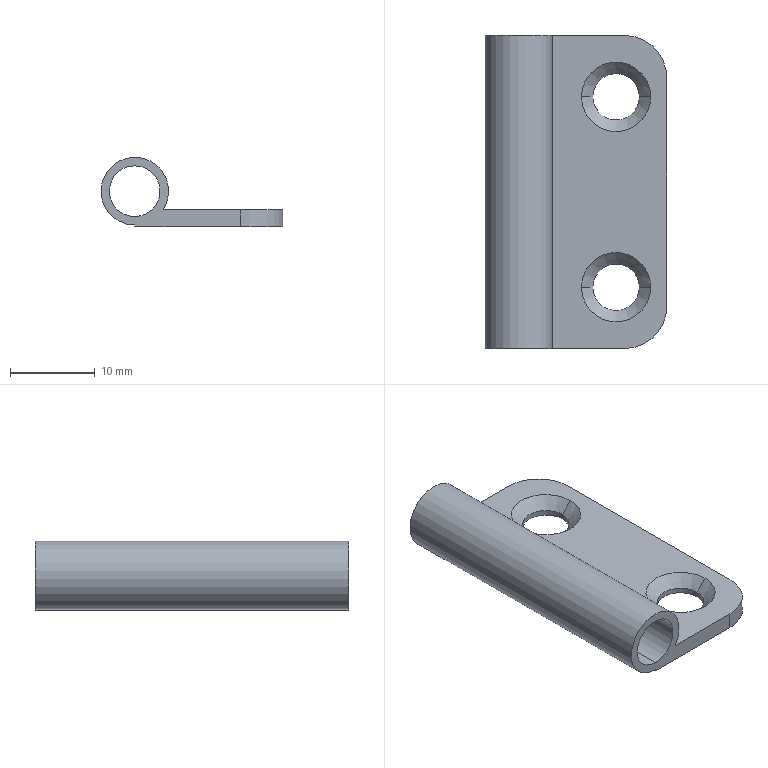Part | STEP file | heye1 | 1 solid | 19 faces | box 21.5 x 37 x 8.2 mm | volume 1799 mm3 | cylinder 9 | plane 6 | cone 4 | commonest cylinder face diameters 5.5 x4 6 x2 10 x2 8 x1
STEP:
#1=CARTESIAN_POINT('',(0.,0.,0.));
#2=DIRECTION('',(0.,0.,1.));
#3=DIRECTION('',(1.,0.,0.));
#4=AXIS2_PLACEMENT_3D('',#1,#2,#3);
#5=CARTESIAN_POINT('',(5.5,11.25,0.65));
#6=VERTEX_POINT('',#5);
#7=CARTESIAN_POINT('',(6.85,11.25,2.));
#8=VERTEX_POINT('',#7);
#9=CARTESIAN_POINT('',(6.85,11.25,2.));
#10=DIRECTION('',(0.7071,0.,0.7071));
#11=VECTOR('',#10,1.);
#12=LINE('',#9,#11);
#13=CARTESIAN_POINT('',(2.75,11.25,2.));
#14=DIRECTION('',(0.,0.,1.));
#15=DIRECTION('',(1.,0.,0.));
#16=AXIS2_PLACEMENT_3D('',#13,#14,#15);
#17=CONICAL_SURFACE('',#16,4.1,0.7854);
#18=CARTESIAN_POINT('',(6.283,0.));
#19=DIRECTION('',(0.,1.));
#20=VECTOR('',#19,1.);
#21=LINE('',#18,#20);
#22=(GEOMETRIC_REPRESENTATION_CONTEXT(2)PARAMETRIC_REPRESENTATION_CONTEXT()REPRESENTATION_CONTEXT('',''));
#23=DEFINITIONAL_REPRESENTATION('',(#21),#22);
#24=PCURVE('',#17,#23);
#25=CARTESIAN_POINT('',(2.75,11.25,2.));
#26=DIRECTION('',(0.,0.,1.));
#27=DIRECTION('',(1.,0.,0.));
#28=AXIS2_PLACEMENT_3D('',#25,#26,#27);
#29=CONICAL_SURFACE('',#28,4.1,0.7854);
#30=CARTESIAN_POINT('',(0.,0.));
#31=DIRECTION('',(0.,1.));
#32=VECTOR('',#31,1.);
#33=LINE('',#30,#32);
#34=(GEOMETRIC_REPRESENTATION_CONTEXT(2)PARAMETRIC_REPRESENTATION_CONTEXT()REPRESENTATION_CONTEXT('',''));
#35=DEFINITIONAL_REPRESENTATION('',(#33),#34);
#36=PCURVE('',#29,#35);
#37=SURFACE_CURVE('',#12,(#24,#36),.PCURVE_S1.);
#38=EDGE_CURVE('',#6,#8,#37,.T.);
#39=ORIENTED_EDGE('',*,*,#38,.T.);
#40=CARTESIAN_POINT('',(-1.35,11.25,2.));
#41=VERTEX_POINT('',#40);
#42=CARTESIAN_POINT('',(2.75,11.25,2.));
#43=DIRECTION('',(0.,0.,1.));
#44=DIRECTION('',(1.,0.,0.));
#45=AXIS2_PLACEMENT_3D('',#42,#43,#44);
#46=CIRCLE('',#45,4.1);
#47=CARTESIAN_POINT('',(0.,0.));
#48=DIRECTION('',(1.,0.));
#49=VECTOR('',#48,1.);
#50=LINE('',#47,#49);
#51=(GEOMETRIC_REPRESENTATION_CONTEXT(2)PARAMETRIC_REPRESENTATION_CONTEXT()REPRESENTATION_CONTEXT('',''));
#52=DEFINITIONAL_REPRESENTATION('',(#50),#51);
#53=PCURVE('',#17,#52);
#54=CARTESIAN_POINT('',(0.,0.,2.));
#55=DIRECTION('',(0.,0.,-1.));
#56=DIRECTION('',(-1.,0.,0.));
#57=AXIS2_PLACEMENT_3D('',#54,#55,#56);
#58=PLANE('',#57);
#59=CARTESIAN_POINT('',(-6.85,11.25));
#60=CARTESIAN_POINT('',(-6.85,18.351));
#61=CARTESIAN_POINT('',(-0.7,14.801));
#62=CARTESIAN_POINT('',(5.45,11.25));
#63=CARTESIAN_POINT('',(-0.7,7.699));
#64=CARTESIAN_POINT('',(-6.85,4.149));
#65=CARTESIAN_POINT('',(-6.85,11.25));
#66=(BOUNDED_CURVE()B_SPLINE_CURVE(2,(#59,#60,#61,#62,#63,#64,#65),.UNSPECIFIED.,.T.,.F.)B_SPLINE_CURVE_WITH_KNOTS((1,2,2,2,2,1),(-2.094,0.,2.094,4.189,6.283,8.378),.UNSPECIFIED.)CURVE()GEOMETRIC_REPRESENTATION_ITEM()RATIONAL_B_SPLINE_CURVE((1.,0.5,1.,0.5,1.,0.5,1.))REPRESENTATION_ITEM(''));
#67=(GEOMETRIC_REPRESENTATION_CONTEXT(2)PARAMETRIC_REPRESENTATION_CONTEXT()REPRESENTATION_CONTEXT('',''));
#68=DEFINITIONAL_REPRESENTATION('',(#66),#67);
#69=PCURVE('',#58,#68);
#70=SURFACE_CURVE('',#46,(#53,#69),.PCURVE_S1.);
#71=EDGE_CURVE('',#41,#8,#70,.T.);
#72=ORIENTED_EDGE('',*,*,#71,.F.);
#73=CARTESIAN_POINT('',(0.,11.25,0.65));
#74=VERTEX_POINT('',#73);
#75=CARTESIAN_POINT('',(-1.35,11.25,2.));
#76=DIRECTION('',(-0.7071,0.,0.7071));
#77=VECTOR('',#76,1.);
#78=LINE('',#75,#77);
#79=CARTESIAN_POINT('',(3.142,0.));
#80=DIRECTION('',(0.,1.));
#81=VECTOR('',#80,1.);
#82=LINE('',#79,#81);
#83=(GEOMETRIC_REPRESENTATION_CONTEXT(2)PARAMETRIC_REPRESENTATION_CONTEXT()REPRESENTATION_CONTEXT('',''));
#84=DEFINITIONAL_REPRESENTATION('',(#82),#83);
#85=PCURVE('',#17,#84);
#86=CARTESIAN_POINT('',(3.142,0.));
#87=DIRECTION('',(0.,1.));
#88=VECTOR('',#87,1.);
#89=LINE('',#86,#88);
#90=(GEOMETRIC_REPRESENTATION_CONTEXT(2)PARAMETRIC_REPRESENTATION_CONTEXT()REPRESENTATION_CONTEXT('',''));
#91=DEFINITIONAL_REPRESENTATION('',(#89),#90);
#92=PCURVE('',#29,#91);
#93=SURFACE_CURVE('',#78,(#85,#92),.PCURVE_S1.);
#94=EDGE_CURVE('',#74,#41,#93,.T.);
#95=ORIENTED_EDGE('',*,*,#94,.F.);
#96=CARTESIAN_POINT('',(2.75,11.25,0.65));
#97=DIRECTION('',(0.,0.,1.));
#98=DIRECTION('',(1.,0.,0.));
#99=AXIS2_PLACEMENT_3D('',#96,#97,#98);
#100=CIRCLE('',#99,2.75);
#101=CARTESIAN_POINT('',(0.,-1.35));
#102=DIRECTION('',(1.,0.));
#103=VECTOR('',#102,1.);
#104=LINE('',#101,#103);
#105=(GEOMETRIC_REPRESENTATION_CONTEXT(2)PARAMETRIC_REPRESENTATION_CONTEXT()REPRESENTATION_CONTEXT('',''));
#106=DEFINITIONAL_REPRESENTATION('',(#104),#105);
#107=PCURVE('',#17,#106);
#108=CARTESIAN_POINT('',(2.75,11.25,2.));
#109=DIRECTION('',(0.,0.,1.));
#110=DIRECTION('',(1.,0.,0.));
#111=AXIS2_PLACEMENT_3D('',#108,#109,#110);
#112=CYLINDRICAL_SURFACE('',#111,2.75);
#113=CARTESIAN_POINT('',(0.,-1.35));
#114=DIRECTION('',(1.,0.));
#115=VECTOR('',#114,1.);
#116=LINE('',#113,#115);
#117=(GEOMETRIC_REPRESENTATION_CONTEXT(2)PARAMETRIC_REPRESENTATION_CONTEXT()REPRESENTATION_CONTEXT('',''));
#118=DEFINITIONAL_REPRESENTATION('',(#116),#117);
#119=PCURVE('',#112,#118);
#120=SURFACE_CURVE('',#100,(#107,#119),.PCURVE_S1.);
#121=EDGE_CURVE('',#74,#6,#120,.T.);
#122=ORIENTED_EDGE('',*,*,#121,.T.);
#123=EDGE_LOOP('',(#39,#72,#95,#122));
#124=FACE_BOUND('',#123,.F.);
#125=ADVANCED_FACE('',(#124),#17,.F.);
#126=CARTESIAN_POINT('',(5.5,11.25,0.));
#127=VERTEX_POINT('',#126);
#128=CARTESIAN_POINT('',(5.5,11.25,2.));
#129=DIRECTION('',(0.,0.,1.));
#130=VECTOR('',#129,1.);
#131=LINE('',#128,#130);
#132=CARTESIAN_POINT('',(6.283,0.));
#133=DIRECTION('',(0.,1.));
#134=VECTOR('',#133,1.);
#135=LINE('',#132,#134);
#136=(GEOMETRIC_REPRESENTATION_CONTEXT(2)PARAMETRIC_REPRESENTATION_CONTEXT()REPRESENTATION_CONTEXT('',''));
#137=DEFINITIONAL_REPRESENTATION('',(#135),#136);
#138=PCURVE('',#112,#137);
#139=CARTESIAN_POINT('',(2.75,11.25,2.));
#140=DIRECTION('',(0.,0.,1.));
#141=DIRECTION('',(1.,0.,0.));
#142=AXIS2_PLACEMENT_3D('',#139,#140,#141);
#143=CYLINDRICAL_SURFACE('',#142,2.75);
#144=CARTESIAN_POINT('',(0.,0.));
#145=DIRECTION('',(0.,1.));
#146=VECTOR('',#145,1.);
#147=LINE('',#144,#146);
#148=(GEOMETRIC_REPRESENTATION_CONTEXT(2)PARAMETRIC_REPRESENTATION_CONTEXT()REPRESENTATION_CONTEXT('',''));
#149=DEFINITIONAL_REPRESENTATION('',(#147),#148);
#150=PCURVE('',#143,#149);
#151=SURFACE_CURVE('',#131,(#138,#150),.PCURVE_S1.);
#152=EDGE_CURVE('',#127,#6,#151,.T.);
#153=ORIENTED_EDGE('',*,*,#152,.T.);
#154=ORIENTED_EDGE('',*,*,#121,.F.);
#155=CARTESIAN_POINT('',(0.,11.25,0.));
#156=VERTEX_POINT('',#155);
#157=CARTESIAN_POINT('',(0.,11.25,2.));
#158=DIRECTION('',(0.,0.,1.));
#159=VECTOR('',#158,1.);
#160=LINE('',#157,#159);
#161=CARTESIAN_POINT('',(3.142,0.));
#162=DIRECTION('',(0.,1.));
#163=VECTOR('',#162,1.);
#164=LINE('',#161,#163);
#165=(GEOMETRIC_REPRESENTATION_CONTEXT(2)PARAMETRIC_REPRESENTATION_CONTEXT()REPRESENTATION_CONTEXT('',''));
#166=DEFINITIONAL_REPRESENTATION('',(#164),#165);
#167=PCURVE('',#112,#166);
#168=CARTESIAN_POINT('',(3.142,0.));
#169=DIRECTION('',(0.,1.));
#170=VECTOR('',#169,1.);
#171=LINE('',#168,#170);
#172=(GEOMETRIC_REPRESENTATION_CONTEXT(2)PARAMETRIC_REPRESENTATION_CONTEXT()REPRESENTATION_CONTEXT('',''));
#173=DEFINITIONAL_REPRESENTATION('',(#171),#172);
#174=PCURVE('',#143,#173);
#175=SURFACE_CURVE('',#160,(#167,#174),.PCURVE_S1.);
#176=EDGE_CURVE('',#156,#74,#175,.T.);
#177=ORIENTED_EDGE('',*,*,#176,.F.);
#178=CARTESIAN_POINT('',(2.75,11.25,0.));
#179=DIRECTION('',(0.,0.,1.));
#180=DIRECTION('',(1.,0.,0.));
#181=AXIS2_PLACEMENT_3D('',#178,#179,#180);
#182=CIRCLE('',#181,2.75);
#183=CARTESIAN_POINT('',(0.,-2.));
#184=DIRECTION('',(1.,0.));
#185=VECTOR('',#184,1.);
#186=LINE('',#183,#185);
#187=(GEOMETRIC_REPRESENTATION_CONTEXT(2)PARAMETRIC_REPRESENTATION_CONTEXT()REPRESENTATION_CONTEXT('',''));
#188=DEFINITIONAL_REPRESENTATION('',(#186),#187);
#189=PCURVE('',#112,#188);
#190=CARTESIAN_POINT('',(0.,0.,0.));
#191=DIRECTION('',(0.,0.,-1.));
#192=DIRECTION('',(-1.,0.,0.));
#193=AXIS2_PLACEMENT_3D('',#190,#191,#192);
#194=PLANE('',#193);
#195=CARTESIAN_POINT('',(-5.5,11.25));
#196=CARTESIAN_POINT('',(-5.5,16.013));
#197=CARTESIAN_POINT('',(-1.375,13.632));
#198=CARTESIAN_POINT('',(2.75,11.25));
#199=CARTESIAN_POINT('',(-1.375,8.868));
#200=CARTESIAN_POINT('',(-5.5,6.487));
#201=CARTESIAN_POINT('',(-5.5,11.25));
#202=(BOUNDED_CURVE()B_SPLINE_CURVE(2,(#195,#196,#197,#198,#199,#200,#201),.UNSPECIFIED.,.T.,.F.)B_SPLINE_CURVE_WITH_KNOTS((1,2,2,2,2,1),(-2.094,0.,2.094,4.189,6.283,8.378),.UNSPECIFIED.)CURVE()GEOMETRIC_REPRESENTATION_ITEM()RATIONAL_B_SPLINE_CURVE((1.,0.5,1.,0.5,1.,0.5,1.))REPRESENTATION_ITEM(''));
#203=(GEOMETRIC_REPRESENTATION_CONTEXT(2)PARAMETRIC_REPRESENTATION_CONTEXT()REPRESENTATION_CONTEXT('',''));
#204=DEFINITIONAL_REPRESENTATION('',(#202),#203);
#205=PCURVE('',#194,#204);
#206=SURFACE_CURVE('',#182,(#189,#205),.PCURVE_S1.);
#207=EDGE_CURVE('',#156,#127,#206,.T.);
#208=ORIENTED_EDGE('',*,*,#207,.T.);
#209=EDGE_LOOP('',(#153,#154,#177,#208));
#210=FACE_BOUND('',#209,.F.);
#211=ADVANCED_FACE('',(#210),#112,.F.);
#212=CARTESIAN_POINT('',(5.5,-11.25,0.65));
#213=VERTEX_POINT('',#212);
#214=CARTESIAN_POINT('',(6.85,-11.25,2.));
#215=VERTEX_POINT('',#214);
#216=CARTESIAN_POINT('',(6.85,-11.25,2.));
#217=DIRECTION('',(0.7071,0.,0.7071));
#218=VECTOR('',#217,1.);
#219=LINE('',#216,#218);
#220=CARTESIAN_POINT('',(2.75,-11.25,2.));
#221=DIRECTION('',(0.,0.,1.));
#222=DIRECTION('',(1.,0.,0.));
#223=AXIS2_PLACEMENT_3D('',#220,#221,#222);
#224=CONICAL_SURFACE('',#223,4.1,0.7854);
#225=CARTESIAN_POINT('',(6.283,0.));
#226=DIRECTION('',(0.,1.));
#227=VECTOR('',#226,1.);
#228=LINE('',#225,#227);
#229=(GEOMETRIC_REPRESENTATION_CONTEXT(2)PARAMETRIC_REPRESENTATION_CONTEXT()REPRESENTATION_CONTEXT('',''));
#230=DEFINITIONAL_REPRESENTATION('',(#228),#229);
#231=PCURVE('',#224,#230);
#232=CARTESIAN_POINT('',(2.75,-11.25,2.));
#233=DIRECTION('',(0.,0.,1.));
#234=DIRECTION('',(1.,0.,0.));
#235=AXIS2_PLACEMENT_3D('',#232,#233,#234);
#236=CONICAL_SURFACE('',#235,4.1,0.7854);
#237=CARTESIAN_POINT('',(0.,0.));
#238=DIRECTION('',(0.,1.));
#239=VECTOR('',#238,1.);
#240=LINE('',#237,#239);
#241=(GEOMETRIC_REPRESENTATION_CONTEXT(2)PARAMETRIC_REPRESENTATION_CONTEXT()REPRESENTATION_CONTEXT('',''));
#242=DEFINITIONAL_REPRESENTATION('',(#240),#241);
#243=PCURVE('',#236,#242);
#244=SURFACE_CURVE('',#219,(#231,#243),.PCURVE_S1.);
#245=EDGE_CURVE('',#213,#215,#244,.T.);
#246=ORIENTED_EDGE('',*,*,#245,.T.);
#247=CARTESIAN_POINT('',(-1.35,-11.25,2.));
#248=VERTEX_POINT('',#247);
#249=CARTESIAN_POINT('',(2.75,-11.25,2.));
#250=DIRECTION('',(0.,0.,1.));
#251=DIRECTION('',(1.,0.,0.));
#252=AXIS2_PLACEMENT_3D('',#249,#250,#251);
#253=CIRCLE('',#252,4.1);
#254=CARTESIAN_POINT('',(0.,0.));
#255=DIRECTION('',(1.,0.));
#256=VECTOR('',#255,1.);
#257=LINE('',#254,#256);
#258=(GEOMETRIC_REPRESENTATION_CONTEXT(2)PARAMETRIC_REPRESENTATION_CONTEXT()REPRESENTATION_CONTEXT('',''));
#259=DEFINITIONAL_REPRESENTATION('',(#257),#258);
#260=PCURVE('',#224,#259);
#261=CARTESIAN_POINT('',(-6.85,-11.25));
#262=CARTESIAN_POINT('',(-6.85,-4.149));
#263=CARTESIAN_POINT('',(-0.7,-7.699));
#264=CARTESIAN_POINT('',(5.45,-11.25));
#265=CARTESIAN_POINT('',(-0.7,-14.801));
#266=CARTESIAN_POINT('',(-6.85,-18.351));
#267=CARTESIAN_POINT('',(-6.85,-11.25));
#268=(BOUNDED_CURVE()B_SPLINE_CURVE(2,(#261,#262,#263,#264,#265,#266,#267),.UNSPECIFIED.,.T.,.F.)B_SPLINE_CURVE_WITH_KNOTS((1,2,2,2,2,1),(-2.094,0.,2.094,4.189,6.283,8.378),.UNSPECIFIED.)CURVE()GEOMETRIC_REPRESENTATION_ITEM()RATIONAL_B_SPLINE_CURVE((1.,0.5,1.,0.5,1.,0.5,1.))REPRESENTATION_ITEM(''));
#269=(GEOMETRIC_REPRESENTATION_CONTEXT(2)PARAMETRIC_REPRESENTATION_CONTEXT()REPRESENTATION_CONTEXT('',''));
#270=DEFINITIONAL_REPRESENTATION('',(#268),#269);
#271=PCURVE('',#58,#270);
#272=SURFACE_CURVE('',#253,(#260,#271),.PCURVE_S1.);
#273=EDGE_CURVE('',#248,#215,#272,.T.);
#274=ORIENTED_EDGE('',*,*,#273,.F.);
#275=CARTESIAN_POINT('',(0.,-11.25,0.65));
#276=VERTEX_POINT('',#275);
#277=CARTESIAN_POINT('',(-1.35,-11.25,2.));
#278=DIRECTION('',(-0.7071,0.,0.7071));
#279=VECTOR('',#278,1.);
#280=LINE('',#277,#279);
#281=CARTESIAN_POINT('',(3.142,0.));
#282=DIRECTION('',(0.,1.));
#283=VECTOR('',#282,1.);
#284=LINE('',#281,#283);
#285=(GEOMETRIC_REPRESENTATION_CONTEXT(2)PARAMETRIC_REPRESENTATION_CONTEXT()REPRESENTATION_CONTEXT('',''));
#286=DEFINITIONAL_REPRESENTATION('',(#284),#285);
#287=PCURVE('',#224,#286);
#288=CARTESIAN_POINT('',(3.142,0.));
#289=DIRECTION('',(0.,1.));
#290=VECTOR('',#289,1.);
#291=LINE('',#288,#290);
#292=(GEOMETRIC_REPRESENTATION_CONTEXT(2)PARAMETRIC_REPRESENTATION_CONTEXT()REPRESENTATION_CONTEXT('',''));
#293=DEFINITIONAL_REPRESENTATION('',(#291),#292);
#294=PCURVE('',#236,#293);
#295=SURFACE_CURVE('',#280,(#287,#294),.PCURVE_S1.);
#296=EDGE_CURVE('',#276,#248,#295,.T.);
#297=ORIENTED_EDGE('',*,*,#296,.F.);
#298=CARTESIAN_POINT('',(2.75,-11.25,0.65));
#299=DIRECTION('',(0.,0.,1.));
#300=DIRECTION('',(1.,0.,0.));
#301=AXIS2_PLACEMENT_3D('',#298,#299,#300);
#302=CIRCLE('',#301,2.75);
#303=CARTESIAN_POINT('',(0.,-1.35));
#304=DIRECTION('',(1.,0.));
#305=VECTOR('',#304,1.);
#306=LINE('',#303,#305);
#307=(GEOMETRIC_REPRESENTATION_CONTEXT(2)PARAMETRIC_REPRESENTATION_CONTEXT()REPRESENTATION_CONTEXT('',''));
#308=DEFINITIONAL_REPRESENTATION('',(#306),#307);
#309=PCURVE('',#224,#308);
#310=CARTESIAN_POINT('',(2.75,-11.25,2.));
#311=DIRECTION('',(0.,0.,1.));
#312=DIRECTION('',(1.,0.,0.));
#313=AXIS2_PLACEMENT_3D('',#310,#311,#312);
#314=CYLINDRICAL_SURFACE('',#313,2.75);
#315=CARTESIAN_POINT('',(0.,-1.35));
#316=DIRECTION('',(1.,0.));
#317=VECTOR('',#316,1.);
#318=LINE('',#315,#317);
#319=(GEOMETRIC_REPRESENTATION_CONTEXT(2)PARAMETRIC_REPRESENTATION_CONTEXT()REPRESENTATION_CONTEXT('',''));
#320=DEFINITIONAL_REPRESENTATION('',(#318),#319);
#321=PCURVE('',#314,#320);
#322=SURFACE_CURVE('',#302,(#309,#321),.PCURVE_S1.);
#323=EDGE_CURVE('',#276,#213,#322,.T.);
#324=ORIENTED_EDGE('',*,*,#323,.T.);
#325=EDGE_LOOP('',(#246,#274,#297,#324));
#326=FACE_BOUND('',#325,.F.);
#327=ADVANCED_FACE('',(#326),#224,.F.);
#328=CARTESIAN_POINT('',(5.5,-11.25,0.));
#329=VERTEX_POINT('',#328);
#330=CARTESIAN_POINT('',(5.5,-11.25,2.));
#331=DIRECTION('',(0.,0.,1.));
#332=VECTOR('',#331,1.);
#333=LINE('',#330,#332);
#334=CARTESIAN_POINT('',(6.283,0.));
#335=DIRECTION('',(0.,1.));
#336=VECTOR('',#335,1.);
#337=LINE('',#334,#336);
#338=(GEOMETRIC_REPRESENTATION_CONTEXT(2)PARAMETRIC_REPRESENTATION_CONTEXT()REPRESENTATION_CONTEXT('',''));
#339=DEFINITIONAL_REPRESENTATION('',(#337),#338);
#340=PCURVE('',#314,#339);
#341=CARTESIAN_POINT('',(2.75,-11.25,2.));
#342=DIRECTION('',(0.,0.,1.));
#343=DIRECTION('',(1.,0.,0.));
#344=AXIS2_PLACEMENT_3D('',#341,#342,#343);
#345=CYLINDRICAL_SURFACE('',#344,2.75);
#346=CARTESIAN_POINT('',(0.,0.));
#347=DIRECTION('',(0.,1.));
#348=VECTOR('',#347,1.);
#349=LINE('',#346,#348);
#350=(GEOMETRIC_REPRESENTATION_CONTEXT(2)PARAMETRIC_REPRESENTATION_CONTEXT()REPRESENTATION_CONTEXT('',''));
#351=DEFINITIONAL_REPRESENTATION('',(#349),#350);
#352=PCURVE('',#345,#351);
#353=SURFACE_CURVE('',#333,(#340,#352),.PCURVE_S1.);
#354=EDGE_CURVE('',#329,#213,#353,.T.);
#355=ORIENTED_EDGE('',*,*,#354,.T.);
#356=ORIENTED_EDGE('',*,*,#323,.F.);
#357=CARTESIAN_POINT('',(0.,-11.25,0.));
#358=VERTEX_POINT('',#357);
#359=CARTESIAN_POINT('',(0.,-11.25,2.));
#360=DIRECTION('',(0.,0.,1.));
#361=VECTOR('',#360,1.);
#362=LINE('',#359,#361);
#363=CARTESIAN_POINT('',(3.142,0.));
#364=DIRECTION('',(0.,1.));
#365=VECTOR('',#364,1.);
#366=LINE('',#363,#365);
#367=(GEOMETRIC_REPRESENTATION_CONTEXT(2)PARAMETRIC_REPRESENTATION_CONTEXT()REPRESENTATION_CONTEXT('',''));
#368=DEFINITIONAL_REPRESENTATION('',(#366),#367);
#369=PCURVE('',#314,#368);
#370=CARTESIAN_POINT('',(3.142,0.));
#371=DIRECTION('',(0.,1.));
#372=VECTOR('',#371,1.);
#373=LINE('',#370,#372);
#374=(GEOMETRIC_REPRESENTATION_CONTEXT(2)PARAMETRIC_REPRESENTATION_CONTEXT()REPRESENTATION_CONTEXT('',''));
#375=DEFINITIONAL_REPRESENTATION('',(#373),#374);
#376=PCURVE('',#345,#375);
#377=SURFACE_CURVE('',#362,(#369,#376),.PCURVE_S1.);
#378=EDGE_CURVE('',#358,#276,#377,.T.);
#379=ORIENTED_EDGE('',*,*,#378,.F.);
#380=CARTESIAN_POINT('',(2.75,-11.25,0.));
#381=DIRECTION('',(0.,0.,1.));
#382=DIRECTION('',(1.,0.,0.));
#383=AXIS2_PLACEMENT_3D('',#380,#381,#382);
#384=CIRCLE('',#383,2.75);
#385=CARTESIAN_POINT('',(0.,-2.));
#386=DIRECTION('',(1.,0.));
#387=VECTOR('',#386,1.);
#388=LINE('',#385,#387);
#389=(GEOMETRIC_REPRESENTATION_CONTEXT(2)PARAMETRIC_REPRESENTATION_CONTEXT()REPRESENTATION_CONTEXT('',''));
#390=DEFINITIONAL_REPRESENTATION('',(#388),#389);
#391=PCURVE('',#314,#390);
#392=CARTESIAN_POINT('',(-5.5,-11.25));
#393=CARTESIAN_POINT('',(-5.5,-6.487));
#394=CARTESIAN_POINT('',(-1.375,-8.868));
#395=CARTESIAN_POINT('',(2.75,-11.25));
#396=CARTESIAN_POINT('',(-1.375,-13.632));
#397=CARTESIAN_POINT('',(-5.5,-16.013));
#398=CARTESIAN_POINT('',(-5.5,-11.25));
#399=(BOUNDED_CURVE()B_SPLINE_CURVE(2,(#392,#393,#394,#395,#396,#397,#398),.UNSPECIFIED.,.T.,.F.)B_SPLINE_CURVE_WITH_KNOTS((1,2,2,2,2,1),(-2.094,0.,2.094,4.189,6.283,8.378),.UNSPECIFIED.)CURVE()GEOMETRIC_REPRESENTATION_ITEM()RATIONAL_B_SPLINE_CURVE((1.,0.5,1.,0.5,1.,0.5,1.))REPRESENTATION_ITEM(''));
#400=(GEOMETRIC_REPRESENTATION_CONTEXT(2)PARAMETRIC_REPRESENTATION_CONTEXT()REPRESENTATION_CONTEXT('',''));
#401=DEFINITIONAL_REPRESENTATION('',(#399),#400);
#402=PCURVE('',#194,#401);
#403=SURFACE_CURVE('',#384,(#391,#402),.PCURVE_S1.);
#404=EDGE_CURVE('',#358,#329,#403,.T.);
#405=ORIENTED_EDGE('',*,*,#404,.T.);
#406=EDGE_LOOP('',(#355,#356,#379,#405));
#407=FACE_BOUND('',#406,.F.);
#408=ADVANCED_FACE('',(#407),#314,.F.);
#409=CARTESIAN_POINT('',(-8.75,-18.5,7.2));
#410=VERTEX_POINT('',#409);
#411=CARTESIAN_POINT('',(-8.75,18.5,7.2));
#412=VERTEX_POINT('',#411);
#413=CARTESIAN_POINT('',(-8.75,-18.5,7.2));
#414=DIRECTION('',(0.,1.,0.));
#415=VECTOR('',#414,1.);
#416=LINE('',#413,#415);
#417=CARTESIAN_POINT('',(-8.75,-18.5,4.2));
#418=DIRECTION('',(0.,1.,0.));
#419=DIRECTION('',(0.,0.,1.));
#420=AXIS2_PLACEMENT_3D('',#417,#418,#419);
#421=CYLINDRICAL_SURFACE('',#420,3.);
#422=CARTESIAN_POINT('',(6.283,0.));
#423=DIRECTION('',(0.,1.));
#424=VECTOR('',#423,1.);
#425=LINE('',#422,#424);
#426=(GEOMETRIC_REPRESENTATION_CONTEXT(2)PARAMETRIC_REPRESENTATION_CONTEXT()REPRESENTATION_CONTEXT('',''));
#427=DEFINITIONAL_REPRESENTATION('',(#425),#426);
#428=PCURVE('',#421,#427);
#429=CARTESIAN_POINT('',(-8.75,-18.5,4.2));
#430=DIRECTION('',(0.,1.,0.));
#431=DIRECTION('',(0.,0.,1.));
#432=AXIS2_PLACEMENT_3D('',#429,#430,#431);
#433=CYLINDRICAL_SURFACE('',#432,3.);
#434=CARTESIAN_POINT('',(0.,0.));
#435=DIRECTION('',(0.,1.));
#436=VECTOR('',#435,1.);
#437=LINE('',#434,#436);
#438=(GEOMETRIC_REPRESENTATION_CONTEXT(2)PARAMETRIC_REPRESENTATION_CONTEXT()REPRESENTATION_CONTEXT('',''));
#439=DEFINITIONAL_REPRESENTATION('',(#437),#438);
#440=PCURVE('',#433,#439);
#441=SURFACE_CURVE('',#416,(#428,#440),.PCURVE_S1.);
#442=EDGE_CURVE('',#410,#412,#441,.T.);
#443=ORIENTED_EDGE('',*,*,#442,.T.);
#444=CARTESIAN_POINT('',(-8.75,18.5,1.2));
#445=VERTEX_POINT('',#444);
#446=CARTESIAN_POINT('',(-8.75,18.5,4.2));
#447=DIRECTION('',(0.,1.,0.));
#448=DIRECTION('',(0.,0.,1.));
#449=AXIS2_PLACEMENT_3D('',#446,#447,#448);
#450=CIRCLE('',#449,3.);
#451=CARTESIAN_POINT('',(0.,37.));
#452=DIRECTION('',(1.,0.));
#453=VECTOR('',#452,1.);
#454=LINE('',#451,#453);
#455=(GEOMETRIC_REPRESENTATION_CONTEXT(2)PARAMETRIC_REPRESENTATION_CONTEXT()REPRESENTATION_CONTEXT('',''));
#456=DEFINITIONAL_REPRESENTATION('',(#454),#455);
#457=PCURVE('',#421,#456);
#458=CARTESIAN_POINT('',(8.75,18.5,2.));
#459=DIRECTION('',(0.,-1.,0.));
#460=DIRECTION('',(1.,0.,0.));
#461=AXIS2_PLACEMENT_3D('',#458,#459,#460);
#462=PLANE('',#461);
#463=CARTESIAN_POINT('',(-17.5,5.2));
#464=CARTESIAN_POINT('',(-12.304,5.2));
#465=CARTESIAN_POINT('',(-14.902,0.7));
#466=CARTESIAN_POINT('',(-17.5,-3.8));
#467=CARTESIAN_POINT('',(-20.098,0.7));
#468=CARTESIAN_POINT('',(-22.696,5.2));
#469=CARTESIAN_POINT('',(-17.5,5.2));
#470=(BOUNDED_CURVE()B_SPLINE_CURVE(2,(#463,#464,#465,#466,#467,#468,#469),.UNSPECIFIED.,.T.,.F.)B_SPLINE_CURVE_WITH_KNOTS((1,2,2,2,2,1),(-2.094,0.,2.094,4.189,6.283,8.378),.UNSPECIFIED.)CURVE()GEOMETRIC_REPRESENTATION_ITEM()RATIONAL_B_SPLINE_CURVE((1.,0.5,1.,0.5,1.,0.5,1.))REPRESENTATION_ITEM(''));
#471=(GEOMETRIC_REPRESENTATION_CONTEXT(2)PARAMETRIC_REPRESENTATION_CONTEXT()REPRESENTATION_CONTEXT('',''));
#472=DEFINITIONAL_REPRESENTATION('',(#470),#471);
#473=PCURVE('',#462,#472);
#474=SURFACE_CURVE('',#450,(#457,#473),.PCURVE_S1.);
#475=EDGE_CURVE('',#445,#412,#474,.T.);
#476=ORIENTED_EDGE('',*,*,#475,.F.);
#477=CARTESIAN_POINT('',(-8.75,-18.5,1.2));
#478=VERTEX_POINT('',#477);
#479=CARTESIAN_POINT('',(-8.75,-18.5,1.2));
#480=DIRECTION('',(0.,1.,0.));
#481=VECTOR('',#480,1.);
#482=LINE('',#479,#481);
#483=CARTESIAN_POINT('',(3.142,0.));
#484=DIRECTION('',(0.,1.));
#485=VECTOR('',#484,1.);
#486=LINE('',#483,#485);
#487=(GEOMETRIC_REPRESENTATION_CONTEXT(2)PARAMETRIC_REPRESENTATION_CONTEXT()REPRESENTATION_CONTEXT('',''));
#488=DEFINITIONAL_REPRESENTATION('',(#486),#487);
#489=PCURVE('',#421,#488);
#490=CARTESIAN_POINT('',(3.142,0.));
#491=DIRECTION('',(0.,1.));
#492=VECTOR('',#491,1.);
#493=LINE('',#490,#492);
#494=(GEOMETRIC_REPRESENTATION_CONTEXT(2)PARAMETRIC_REPRESENTATION_CONTEXT()REPRESENTATION_CONTEXT('',''));
#495=DEFINITIONAL_REPRESENTATION('',(#493),#494);
#496=PCURVE('',#433,#495);
#497=SURFACE_CURVE('',#482,(#489,#496),.PCURVE_S1.);
#498=EDGE_CURVE('',#478,#445,#497,.T.);
#499=ORIENTED_EDGE('',*,*,#498,.F.);
#500=CARTESIAN_POINT('',(-8.75,-18.5,4.2));
#501=DIRECTION('',(0.,1.,0.));
#502=DIRECTION('',(0.,0.,1.));
#503=AXIS2_PLACEMENT_3D('',#500,#501,#502);
#504=CIRCLE('',#503,3.);
#505=CARTESIAN_POINT('',(0.,0.));
#506=DIRECTION('',(1.,0.));
#507=VECTOR('',#506,1.);
#508=LINE('',#505,#507);
#509=(GEOMETRIC_REPRESENTATION_CONTEXT(2)PARAMETRIC_REPRESENTATION_CONTEXT()REPRESENTATION_CONTEXT('',''));
#510=DEFINITIONAL_REPRESENTATION('',(#508),#509);
#511=PCURVE('',#421,#510);
#512=CARTESIAN_POINT('',(8.75,-18.5,2.));
#513=DIRECTION('',(0.,1.,0.));
#514=DIRECTION('',(-1.,0.,0.));
#515=AXIS2_PLACEMENT_3D('',#512,#513,#514);
#516=PLANE('',#515);
#517=CARTESIAN_POINT('',(17.5,2.2));
#518=DIRECTION('',(0.,1.));
#519=AXIS2_PLACEMENT_2D('',#517,#518);
#520=CIRCLE('',#519,3.);
#521=(GEOMETRIC_REPRESENTATION_CONTEXT(2)PARAMETRIC_REPRESENTATION_CONTEXT()REPRESENTATION_CONTEXT('',''));
#522=DEFINITIONAL_REPRESENTATION('',(#520),#521);
#523=PCURVE('',#516,#522);
#524=SURFACE_CURVE('',#504,(#511,#523),.PCURVE_S1.);
#525=EDGE_CURVE('',#478,#410,#524,.T.);
#526=ORIENTED_EDGE('',*,*,#525,.T.);
#527=EDGE_LOOP('',(#443,#476,#499,#526));
#528=FACE_BOUND('',#527,.F.);
#529=ADVANCED_FACE('',(#528),#421,.F.);
#530=CARTESIAN_POINT('',(-8.75,-18.5,0.2));
#531=VERTEX_POINT('',#530);
#532=CARTESIAN_POINT('',(-8.75,-18.5,0.));
#533=VERTEX_POINT('',#532);
#534=CARTESIAN_POINT('',(-8.75,-18.5,2.));
#535=DIRECTION('',(0.,0.,-1.));
#536=VECTOR('',#535,1.);
#537=LINE('',#534,#536);
#538=CARTESIAN_POINT('',(-8.75,18.5,2.));
#539=DIRECTION('',(1.,0.,0.));
#540=DIRECTION('',(0.,1.,0.));
#541=AXIS2_PLACEMENT_3D('',#538,#539,#540);
#542=PLANE('',#541);
#543=CARTESIAN_POINT('',(-37.,0.));
#544=DIRECTION('',(0.,-1.));
#545=VECTOR('',#544,1.);
#546=LINE('',#543,#545);
#547=(GEOMETRIC_REPRESENTATION_CONTEXT(2)PARAMETRIC_REPRESENTATION_CONTEXT()REPRESENTATION_CONTEXT('',''));
#548=DEFINITIONAL_REPRESENTATION('',(#546),#547);
#549=PCURVE('',#542,#548);
#550=CARTESIAN_POINT('',(17.5,0.));
#551=DIRECTION('',(0.,-1.));
#552=VECTOR('',#551,1.);
#553=LINE('',#550,#552);
#554=(GEOMETRIC_REPRESENTATION_CONTEXT(2)PARAMETRIC_REPRESENTATION_CONTEXT()REPRESENTATION_CONTEXT('',''));
#555=DEFINITIONAL_REPRESENTATION('',(#553),#554);
#556=PCURVE('',#516,#555);
#557=SURFACE_CURVE('',#537,(#549,#556),.PCURVE_S1.);
#558=EDGE_CURVE('',#531,#533,#557,.T.);
#559=ORIENTED_EDGE('',*,*,#558,.F.);
#560=CARTESIAN_POINT('',(-8.75,18.5,0.2));
#561=VERTEX_POINT('',#560);
#562=CARTESIAN_POINT('',(-8.75,29.814,0.2));
#563=DIRECTION('',(0.,1.,0.));
#564=VECTOR('',#563,1.);
#565=LINE('',#562,#564);
#566=CARTESIAN_POINT('',(11.314,-1.8));
#567=DIRECTION('',(1.,0.));
#568=VECTOR('',#567,1.);
#569=LINE('',#566,#568);
#570=(GEOMETRIC_REPRESENTATION_CONTEXT(2)PARAMETRIC_REPRESENTATION_CONTEXT()REPRESENTATION_CONTEXT('',''));
#571=DEFINITIONAL_REPRESENTATION('',(#569),#570);
#572=PCURVE('',#542,#571);
#573=CARTESIAN_POINT('',(-8.75,29.814,4.2));
#574=DIRECTION('',(0.,-1.,0.));
#575=DIRECTION('',(0.,0.,-1.));
#576=AXIS2_PLACEMENT_3D('',#573,#574,#575);
#577=CYLINDRICAL_SURFACE('',#576,4.);
#578=CARTESIAN_POINT('',(6.283,0.));
#579=DIRECTION('',(0.,-1.));
#580=VECTOR('',#579,1.);
#581=LINE('',#578,#580);
#582=(GEOMETRIC_REPRESENTATION_CONTEXT(2)PARAMETRIC_REPRESENTATION_CONTEXT()REPRESENTATION_CONTEXT('',''));
#583=DEFINITIONAL_REPRESENTATION('',(#581),#582);
#584=PCURVE('',#577,#583);
#585=SURFACE_CURVE('',#565,(#572,#584),.PCURVE_S1.);
#586=EDGE_CURVE('',#531,#561,#585,.T.);
#587=ORIENTED_EDGE('',*,*,#586,.T.);
#588=CARTESIAN_POINT('',(-8.75,18.5,0.));
#589=VERTEX_POINT('',#588);
#590=CARTESIAN_POINT('',(-8.75,18.5,2.));
#591=DIRECTION('',(0.,0.,-1.));
#592=VECTOR('',#591,1.);
#593=LINE('',#590,#592);
#594=CARTESIAN_POINT('',(0.,0.));
#595=DIRECTION('',(0.,-1.));
#596=VECTOR('',#595,1.);
#597=LINE('',#594,#596);
#598=(GEOMETRIC_REPRESENTATION_CONTEXT(2)PARAMETRIC_REPRESENTATION_CONTEXT()REPRESENTATION_CONTEXT('',''));
#599=DEFINITIONAL_REPRESENTATION('',(#597),#598);
#600=PCURVE('',#542,#599);
#601=CARTESIAN_POINT('',(-17.5,0.));
#602=DIRECTION('',(0.,-1.));
#603=VECTOR('',#602,1.);
#604=LINE('',#601,#603);
#605=(GEOMETRIC_REPRESENTATION_CONTEXT(2)PARAMETRIC_REPRESENTATION_CONTEXT()REPRESENTATION_CONTEXT('',''));
#606=DEFINITIONAL_REPRESENTATION('',(#604),#605);
#607=PCURVE('',#462,#606);
#608=SURFACE_CURVE('',#593,(#600,#607),.PCURVE_S1.);
#609=EDGE_CURVE('',#561,#589,#608,.T.);
#610=ORIENTED_EDGE('',*,*,#609,.T.);
#611=CARTESIAN_POINT('',(-8.75,18.5,0.));
#612=DIRECTION('',(0.,-1.,0.));
#613=VECTOR('',#612,1.);
#614=LINE('',#611,#613);
#615=CARTESIAN_POINT('',(0.,-2.));
#616=DIRECTION('',(-1.,0.));
#617=VECTOR('',#616,1.);
#618=LINE('',#615,#617);
#619=(GEOMETRIC_REPRESENTATION_CONTEXT(2)PARAMETRIC_REPRESENTATION_CONTEXT()REPRESENTATION_CONTEXT('',''));
#620=DEFINITIONAL_REPRESENTATION('',(#618),#619);
#621=PCURVE('',#542,#620);
#622=CARTESIAN_POINT('',(8.75,18.5));
#623=DIRECTION('',(0.,-1.));
#624=VECTOR('',#623,1.);
#625=LINE('',#622,#624);
#626=(GEOMETRIC_REPRESENTATION_CONTEXT(2)PARAMETRIC_REPRESENTATION_CONTEXT()REPRESENTATION_CONTEXT('',''));
#627=DEFINITIONAL_REPRESENTATION('',(#625),#626);
#628=PCURVE('',#194,#627);
#629=SURFACE_CURVE('',#614,(#621,#628),.PCURVE_S1.);
#630=EDGE_CURVE('',#589,#533,#629,.T.);
#631=ORIENTED_EDGE('',*,*,#630,.T.);
#632=EDGE_LOOP('',(#559,#587,#610,#631));
#633=FACE_BOUND('',#632,.T.);
#634=ADVANCED_FACE('',(#633),#542,.F.);
#635=CARTESIAN_POINT('',(-8.75,-18.5,4.2));
#636=DIRECTION('',(0.,1.,0.));
#637=DIRECTION('',(0.,0.,1.));
#638=AXIS2_PLACEMENT_3D('',#635,#636,#637);
#639=CIRCLE('',#638,3.);
#640=CARTESIAN_POINT('',(17.5,2.2));
#641=DIRECTION('',(0.,1.));
#642=AXIS2_PLACEMENT_2D('',#640,#641);
#643=CIRCLE('',#642,3.);
#644=(GEOMETRIC_REPRESENTATION_CONTEXT(2)PARAMETRIC_REPRESENTATION_CONTEXT()REPRESENTATION_CONTEXT('',''));
#645=DEFINITIONAL_REPRESENTATION('',(#643),#644);
#646=PCURVE('',#516,#645);
#647=CARTESIAN_POINT('',(0.,0.));
#648=DIRECTION('',(1.,0.));
#649=VECTOR('',#648,1.);
#650=LINE('',#647,#649);
#651=(GEOMETRIC_REPRESENTATION_CONTEXT(2)PARAMETRIC_REPRESENTATION_CONTEXT()REPRESENTATION_CONTEXT('',''));
#652=DEFINITIONAL_REPRESENTATION('',(#650),#651);
#653=PCURVE('',#433,#652);
#654=SURFACE_CURVE('',#639,(#646,#653),.PCURVE_S1.);
#655=EDGE_CURVE('',#410,#478,#654,.T.);
#656=ORIENTED_EDGE('',*,*,#655,.T.);
#657=ORIENTED_EDGE('',*,*,#525,.T.);
#658=EDGE_LOOP('',(#656,#657));
#659=FACE_BOUND('',#658,.T.);
#660=CARTESIAN_POINT('',(3.75,-18.5,0.));
#661=VERTEX_POINT('',#660);
#662=CARTESIAN_POINT('',(8.75,-18.5,0.));
#663=DIRECTION('',(1.,0.,0.));
#664=VECTOR('',#663,1.);
#665=LINE('',#662,#664);
#666=CARTESIAN_POINT('',(0.,-2.));
#667=DIRECTION('',(-1.,0.));
#668=VECTOR('',#667,1.);
#669=LINE('',#666,#668);
#670=(GEOMETRIC_REPRESENTATION_CONTEXT(2)PARAMETRIC_REPRESENTATION_CONTEXT()REPRESENTATION_CONTEXT('',''));
#671=DEFINITIONAL_REPRESENTATION('',(#669),#670);
#672=PCURVE('',#516,#671);
#673=CARTESIAN_POINT('',(-8.75,-18.5));
#674=DIRECTION('',(-1.,0.));
#675=VECTOR('',#674,1.);
#676=LINE('',#673,#675);
#677=(GEOMETRIC_REPRESENTATION_CONTEXT(2)PARAMETRIC_REPRESENTATION_CONTEXT()REPRESENTATION_CONTEXT('',''));
#678=DEFINITIONAL_REPRESENTATION('',(#676),#677);
#679=PCURVE('',#194,#678);
#680=SURFACE_CURVE('',#665,(#672,#679),.PCURVE_S1.);
#681=EDGE_CURVE('',#533,#661,#680,.T.);
#682=ORIENTED_EDGE('',*,*,#681,.T.);
#683=CARTESIAN_POINT('',(3.75,-18.5,2.));
#684=VERTEX_POINT('',#683);
#685=CARTESIAN_POINT('',(3.75,-18.5,2.));
#686=DIRECTION('',(0.,0.,1.));
#687=VECTOR('',#686,1.);
#688=LINE('',#685,#687);
#689=CARTESIAN_POINT('',(5.,0.));
#690=DIRECTION('',(0.,1.));
#691=VECTOR('',#690,1.);
#692=LINE('',#689,#691);
#693=(GEOMETRIC_REPRESENTATION_CONTEXT(2)PARAMETRIC_REPRESENTATION_CONTEXT()REPRESENTATION_CONTEXT('',''));
#694=DEFINITIONAL_REPRESENTATION('',(#692),#693);
#695=PCURVE('',#516,#694);
#696=CARTESIAN_POINT('',(3.75,-13.5,2.));
#697=DIRECTION('',(0.,0.,-1.));
#698=DIRECTION('',(-1.,0.,0.));
#699=AXIS2_PLACEMENT_3D('',#696,#697,#698);
#700=CYLINDRICAL_SURFACE('',#699,5.);
#701=CARTESIAN_POINT('',(4.712,0.));
#702=DIRECTION('',(0.,-1.));
#703=VECTOR('',#702,1.);
#704=LINE('',#701,#703);
#705=(GEOMETRIC_REPRESENTATION_CONTEXT(2)PARAMETRIC_REPRESENTATION_CONTEXT()REPRESENTATION_CONTEXT('',''));
#706=DEFINITIONAL_REPRESENTATION('',(#704),#705);
#707=PCURVE('',#700,#706);
#708=SURFACE_CURVE('',#688,(#695,#707),.PCURVE_S1.);
#709=EDGE_CURVE('',#661,#684,#708,.T.);
#710=ORIENTED_EDGE('',*,*,#709,.T.);
#711=CARTESIAN_POINT('',(-5.409,-18.5,2.));
#712=VERTEX_POINT('',#711);
#713=CARTESIAN_POINT('',(8.75,-18.5,2.));
#714=DIRECTION('',(1.,0.,0.));
#715=VECTOR('',#714,1.);
#716=LINE('',#713,#715);
#717=CARTESIAN_POINT('',(0.,0.));
#718=DIRECTION('',(-1.,0.));
#719=VECTOR('',#718,1.);
#720=LINE('',#717,#719);
#721=(GEOMETRIC_REPRESENTATION_CONTEXT(2)PARAMETRIC_REPRESENTATION_CONTEXT()REPRESENTATION_CONTEXT('',''));
#722=DEFINITIONAL_REPRESENTATION('',(#720),#721);
#723=PCURVE('',#516,#722);
#724=CARTESIAN_POINT('',(-8.75,-18.5));
#725=DIRECTION('',(-1.,0.));
#726=VECTOR('',#725,1.);
#727=LINE('',#724,#726);
#728=(GEOMETRIC_REPRESENTATION_CONTEXT(2)PARAMETRIC_REPRESENTATION_CONTEXT()REPRESENTATION_CONTEXT('',''));
#729=DEFINITIONAL_REPRESENTATION('',(#727),#728);
#730=PCURVE('',#58,#729);
#731=SURFACE_CURVE('',#716,(#723,#730),.PCURVE_S1.);
#732=EDGE_CURVE('',#712,#684,#731,.T.);
#733=ORIENTED_EDGE('',*,*,#732,.F.);
#734=CARTESIAN_POINT('',(-8.75,-18.5,4.2));
#735=DIRECTION('',(0.,-1.,0.));
#736=DIRECTION('',(0.,0.,-1.));
#737=AXIS2_PLACEMENT_3D('',#734,#735,#736);
#738=CIRCLE('',#737,4.);
#739=CARTESIAN_POINT('',(17.5,-1.8));
#740=CARTESIAN_POINT('',(10.572,-1.8));
#741=CARTESIAN_POINT('',(14.036,4.2));
#742=CARTESIAN_POINT('',(17.5,10.2));
#743=CARTESIAN_POINT('',(20.964,4.2));
#744=CARTESIAN_POINT('',(24.428,-1.8));
#745=CARTESIAN_POINT('',(17.5,-1.8));
#746=(BOUNDED_CURVE()B_SPLINE_CURVE(2,(#739,#740,#741,#742,#743,#744,#745),.UNSPECIFIED.,.T.,.F.)B_SPLINE_CURVE_WITH_KNOTS((1,2,2,2,2,1),(-2.094,0.,2.094,4.189,6.283,8.378),.UNSPECIFIED.)CURVE()GEOMETRIC_REPRESENTATION_ITEM()RATIONAL_B_SPLINE_CURVE((1.,0.5,1.,0.5,1.,0.5,1.))REPRESENTATION_ITEM(''));
#747=(GEOMETRIC_REPRESENTATION_CONTEXT(2)PARAMETRIC_REPRESENTATION_CONTEXT()REPRESENTATION_CONTEXT('',''));
#748=DEFINITIONAL_REPRESENTATION('',(#746),#747);
#749=PCURVE('',#516,#748);
#750=CARTESIAN_POINT('',(0.,48.314));
#751=DIRECTION('',(1.,0.));
#752=VECTOR('',#751,1.);
#753=LINE('',#750,#752);
#754=(GEOMETRIC_REPRESENTATION_CONTEXT(2)PARAMETRIC_REPRESENTATION_CONTEXT()REPRESENTATION_CONTEXT('',''));
#755=DEFINITIONAL_REPRESENTATION('',(#753),#754);
#756=PCURVE('',#577,#755);
#757=SURFACE_CURVE('',#738,(#749,#756),.PCURVE_S1.);
#758=EDGE_CURVE('',#712,#531,#757,.T.);
#759=ORIENTED_EDGE('',*,*,#758,.T.);
#760=ORIENTED_EDGE('',*,*,#558,.T.);
#761=EDGE_LOOP('',(#682,#710,#733,#759,#760));
#762=FACE_BOUND('',#761,.T.);
#763=ADVANCED_FACE('',(#659,#762),#516,.F.);
#764=CARTESIAN_POINT('',(8.75,-13.5,2.));
#765=VERTEX_POINT('',#764);
#766=CARTESIAN_POINT('',(8.75,13.5,2.));
#767=VERTEX_POINT('',#766);
#768=CARTESIAN_POINT('',(8.75,18.5,2.));
#769=DIRECTION('',(0.,1.,0.));
#770=VECTOR('',#769,1.);
#771=LINE('',#768,#770);
#772=CARTESIAN_POINT('',(8.75,18.5,2.));
#773=DIRECTION('',(-1.,0.,0.));
#774=DIRECTION('',(0.,-1.,0.));
#775=AXIS2_PLACEMENT_3D('',#772,#773,#774);
#776=PLANE('',#775);
#777=CARTESIAN_POINT('',(0.,0.));
#778=DIRECTION('',(-1.,0.));
#779=VECTOR('',#778,1.);
#780=LINE('',#777,#779);
#781=(GEOMETRIC_REPRESENTATION_CONTEXT(2)PARAMETRIC_REPRESENTATION_CONTEXT()REPRESENTATION_CONTEXT('',''));
#782=DEFINITIONAL_REPRESENTATION('',(#780),#781);
#783=PCURVE('',#776,#782);
#784=CARTESIAN_POINT('',(-8.75,18.5));
#785=DIRECTION('',(0.,1.));
#786=VECTOR('',#785,1.);
#787=LINE('',#784,#786);
#788=(GEOMETRIC_REPRESENTATION_CONTEXT(2)PARAMETRIC_REPRESENTATION_CONTEXT()REPRESENTATION_CONTEXT('',''));
#789=DEFINITIONAL_REPRESENTATION('',(#787),#788);
#790=PCURVE('',#58,#789);
#791=SURFACE_CURVE('',#771,(#783,#790),.PCURVE_S1.);
#792=EDGE_CURVE('',#765,#767,#791,.T.);
#793=ORIENTED_EDGE('',*,*,#792,.F.);
#794=CARTESIAN_POINT('',(8.75,-13.5,0.));
#795=VERTEX_POINT('',#794);
#796=CARTESIAN_POINT('',(8.75,-13.5,2.));
#797=DIRECTION('',(0.,0.,-1.));
#798=VECTOR('',#797,1.);
#799=LINE('',#796,#798);
#800=CARTESIAN_POINT('',(32.,0.));
#801=DIRECTION('',(0.,-1.));
#802=VECTOR('',#801,1.);
#803=LINE('',#800,#802);
#804=(GEOMETRIC_REPRESENTATION_CONTEXT(2)PARAMETRIC_REPRESENTATION_CONTEXT()REPRESENTATION_CONTEXT('',''));
#805=DEFINITIONAL_REPRESENTATION('',(#803),#804);
#806=PCURVE('',#776,#805);
#807=CARTESIAN_POINT('',(3.142,0.));
#808=DIRECTION('',(0.,1.));
#809=VECTOR('',#808,1.);
#810=LINE('',#807,#809);
#811=(GEOMETRIC_REPRESENTATION_CONTEXT(2)PARAMETRIC_REPRESENTATION_CONTEXT()REPRESENTATION_CONTEXT('',''));
#812=DEFINITIONAL_REPRESENTATION('',(#810),#811);
#813=PCURVE('',#700,#812);
#814=SURFACE_CURVE('',#799,(#806,#813),.PCURVE_S1.);
#815=EDGE_CURVE('',#765,#795,#814,.T.);
#816=ORIENTED_EDGE('',*,*,#815,.T.);
#817=CARTESIAN_POINT('',(8.75,13.5,0.));
#818=VERTEX_POINT('',#817);
#819=CARTESIAN_POINT('',(8.75,18.5,0.));
#820=DIRECTION('',(0.,1.,0.));
#821=VECTOR('',#820,1.);
#822=LINE('',#819,#821);
#823=CARTESIAN_POINT('',(0.,-2.));
#824=DIRECTION('',(-1.,0.));
#825=VECTOR('',#824,1.);
#826=LINE('',#823,#825);
#827=(GEOMETRIC_REPRESENTATION_CONTEXT(2)PARAMETRIC_REPRESENTATION_CONTEXT()REPRESENTATION_CONTEXT('',''));
#828=DEFINITIONAL_REPRESENTATION('',(#826),#827);
#829=PCURVE('',#776,#828);
#830=CARTESIAN_POINT('',(-8.75,18.5));
#831=DIRECTION('',(0.,1.));
#832=VECTOR('',#831,1.);
#833=LINE('',#830,#832);
#834=(GEOMETRIC_REPRESENTATION_CONTEXT(2)PARAMETRIC_REPRESENTATION_CONTEXT()REPRESENTATION_CONTEXT('',''));
#835=DEFINITIONAL_REPRESENTATION('',(#833),#834);
#836=PCURVE('',#194,#835);
#837=SURFACE_CURVE('',#822,(#829,#836),.PCURVE_S1.);
#838=EDGE_CURVE('',#795,#818,#837,.T.);
#839=ORIENTED_EDGE('',*,*,#838,.T.);
#840=CARTESIAN_POINT('',(8.75,13.5,2.));
#841=DIRECTION('',(0.,0.,1.));
#842=VECTOR('',#841,1.);
#843=LINE('',#840,#842);
#844=CARTESIAN_POINT('',(5.,0.));
#845=DIRECTION('',(0.,1.));
#846=VECTOR('',#845,1.);
#847=LINE('',#844,#846);
#848=(GEOMETRIC_REPRESENTATION_CONTEXT(2)PARAMETRIC_REPRESENTATION_CONTEXT()REPRESENTATION_CONTEXT('',''));
#849=DEFINITIONAL_REPRESENTATION('',(#847),#848);
#850=PCURVE('',#776,#849);
#851=CARTESIAN_POINT('',(3.75,13.5,2.));
#852=DIRECTION('',(0.,0.,-1.));
#853=DIRECTION('',(-1.,0.,0.));
#854=AXIS2_PLACEMENT_3D('',#851,#852,#853);
#855=CYLINDRICAL_SURFACE('',#854,5.);
#856=CARTESIAN_POINT('',(3.142,0.));
#857=DIRECTION('',(0.,-1.));
#858=VECTOR('',#857,1.);
#859=LINE('',#856,#858);
#860=(GEOMETRIC_REPRESENTATION_CONTEXT(2)PARAMETRIC_REPRESENTATION_CONTEXT()REPRESENTATION_CONTEXT('',''));
#861=DEFINITIONAL_REPRESENTATION('',(#859),#860);
#862=PCURVE('',#855,#861);
#863=SURFACE_CURVE('',#843,(#850,#862),.PCURVE_S1.);
#864=EDGE_CURVE('',#818,#767,#863,.T.);
#865=ORIENTED_EDGE('',*,*,#864,.T.);
#866=EDGE_LOOP('',(#793,#816,#839,#865));
#867=FACE_BOUND('',#866,.T.);
#868=ADVANCED_FACE('',(#867),#776,.F.);
#869=CARTESIAN_POINT('',(-8.75,18.5,4.2));
#870=DIRECTION('',(0.,1.,0.));
#871=DIRECTION('',(0.,0.,1.));
#872=AXIS2_PLACEMENT_3D('',#869,#870,#871);
#873=CIRCLE('',#872,3.);
#874=CARTESIAN_POINT('',(-17.5,5.2));
#875=CARTESIAN_POINT('',(-12.304,5.2));
#876=CARTESIAN_POINT('',(-14.902,0.7));
#877=CARTESIAN_POINT('',(-17.5,-3.8));
#878=CARTESIAN_POINT('',(-20.098,0.7));
#879=CARTESIAN_POINT('',(-22.696,5.2));
#880=CARTESIAN_POINT('',(-17.5,5.2));
#881=(BOUNDED_CURVE()B_SPLINE_CURVE(2,(#874,#875,#876,#877,#878,#879,#880),.UNSPECIFIED.,.T.,.F.)B_SPLINE_CURVE_WITH_KNOTS((1,2,2,2,2,1),(-2.094,0.,2.094,4.189,6.283,8.378),.UNSPECIFIED.)CURVE()GEOMETRIC_REPRESENTATION_ITEM()RATIONAL_B_SPLINE_CURVE((1.,0.5,1.,0.5,1.,0.5,1.))REPRESENTATION_ITEM(''));
#882=(GEOMETRIC_REPRESENTATION_CONTEXT(2)PARAMETRIC_REPRESENTATION_CONTEXT()REPRESENTATION_CONTEXT('',''));
#883=DEFINITIONAL_REPRESENTATION('',(#881),#882);
#884=PCURVE('',#462,#883);
#885=CARTESIAN_POINT('',(0.,37.));
#886=DIRECTION('',(1.,0.));
#887=VECTOR('',#886,1.);
#888=LINE('',#885,#887);
#889=(GEOMETRIC_REPRESENTATION_CONTEXT(2)PARAMETRIC_REPRESENTATION_CONTEXT()REPRESENTATION_CONTEXT('',''));
#890=DEFINITIONAL_REPRESENTATION('',(#888),#889);
#891=PCURVE('',#433,#890);
#892=SURFACE_CURVE('',#873,(#884,#891),.PCURVE_S1.);
#893=EDGE_CURVE('',#412,#445,#892,.T.);
#894=ORIENTED_EDGE('',*,*,#893,.F.);
#895=ORIENTED_EDGE('',*,*,#475,.F.);
#896=EDGE_LOOP('',(#894,#895));
#897=FACE_BOUND('',#896,.T.);
#898=CARTESIAN_POINT('',(3.75,18.5,2.));
#899=VERTEX_POINT('',#898);
#900=CARTESIAN_POINT('',(-5.409,18.5,2.));
#901=VERTEX_POINT('',#900);
#902=CARTESIAN_POINT('',(8.75,18.5,2.));
#903=DIRECTION('',(-1.,0.,0.));
#904=VECTOR('',#903,1.);
#905=LINE('',#902,#904);
#906=CARTESIAN_POINT('',(0.,0.));
#907=DIRECTION('',(-1.,0.));
#908=VECTOR('',#907,1.);
#909=LINE('',#906,#908);
#910=(GEOMETRIC_REPRESENTATION_CONTEXT(2)PARAMETRIC_REPRESENTATION_CONTEXT()REPRESENTATION_CONTEXT('',''));
#911=DEFINITIONAL_REPRESENTATION('',(#909),#910);
#912=PCURVE('',#462,#911);
#913=CARTESIAN_POINT('',(-8.75,18.5));
#914=DIRECTION('',(1.,0.));
#915=VECTOR('',#914,1.);
#916=LINE('',#913,#915);
#917=(GEOMETRIC_REPRESENTATION_CONTEXT(2)PARAMETRIC_REPRESENTATION_CONTEXT()REPRESENTATION_CONTEXT('',''));
#918=DEFINITIONAL_REPRESENTATION('',(#916),#917);
#919=PCURVE('',#58,#918);
#920=SURFACE_CURVE('',#905,(#912,#919),.PCURVE_S1.);
#921=EDGE_CURVE('',#899,#901,#920,.T.);
#922=ORIENTED_EDGE('',*,*,#921,.F.);
#923=CARTESIAN_POINT('',(3.75,18.5,0.));
#924=VERTEX_POINT('',#923);
#925=CARTESIAN_POINT('',(3.75,18.5,2.));
#926=DIRECTION('',(0.,0.,-1.));
#927=VECTOR('',#926,1.);
#928=LINE('',#925,#927);
#929=CARTESIAN_POINT('',(-5.,0.));
#930=DIRECTION('',(0.,-1.));
#931=VECTOR('',#930,1.);
#932=LINE('',#929,#931);
#933=(GEOMETRIC_REPRESENTATION_CONTEXT(2)PARAMETRIC_REPRESENTATION_CONTEXT()REPRESENTATION_CONTEXT('',''));
#934=DEFINITIONAL_REPRESENTATION('',(#932),#933);
#935=PCURVE('',#462,#934);
#936=CARTESIAN_POINT('',(1.571,0.));
#937=DIRECTION('',(0.,1.));
#938=VECTOR('',#937,1.);
#939=LINE('',#936,#938);
#940=(GEOMETRIC_REPRESENTATION_CONTEXT(2)PARAMETRIC_REPRESENTATION_CONTEXT()REPRESENTATION_CONTEXT('',''));
#941=DEFINITIONAL_REPRESENTATION('',(#939),#940);
#942=PCURVE('',#855,#941);
#943=SURFACE_CURVE('',#928,(#935,#942),.PCURVE_S1.);
#944=EDGE_CURVE('',#899,#924,#943,.T.);
#945=ORIENTED_EDGE('',*,*,#944,.T.);
#946=CARTESIAN_POINT('',(8.75,18.5,0.));
#947=DIRECTION('',(-1.,0.,0.));
#948=VECTOR('',#947,1.);
#949=LINE('',#946,#948);
#950=CARTESIAN_POINT('',(0.,-2.));
#951=DIRECTION('',(-1.,0.));
#952=VECTOR('',#951,1.);
#953=LINE('',#950,#952);
#954=(GEOMETRIC_REPRESENTATION_CONTEXT(2)PARAMETRIC_REPRESENTATION_CONTEXT()REPRESENTATION_CONTEXT('',''));
#955=DEFINITIONAL_REPRESENTATION('',(#953),#954);
#956=PCURVE('',#462,#955);
#957=CARTESIAN_POINT('',(-8.75,18.5));
#958=DIRECTION('',(1.,0.));
#959=VECTOR('',#958,1.);
#960=LINE('',#957,#959);
#961=(GEOMETRIC_REPRESENTATION_CONTEXT(2)PARAMETRIC_REPRESENTATION_CONTEXT()REPRESENTATION_CONTEXT('',''));
#962=DEFINITIONAL_REPRESENTATION('',(#960),#961);
#963=PCURVE('',#194,#962);
#964=SURFACE_CURVE('',#949,(#956,#963),.PCURVE_S1.);
#965=EDGE_CURVE('',#924,#589,#964,.T.);
#966=ORIENTED_EDGE('',*,*,#965,.T.);
#967=ORIENTED_EDGE('',*,*,#609,.F.);
#968=CARTESIAN_POINT('',(-8.75,18.5,4.2));
#969=DIRECTION('',(0.,1.,0.));
#970=DIRECTION('',(1.,0.,0.));
#971=AXIS2_PLACEMENT_3D('',#968,#969,#970);
#972=CIRCLE('',#971,4.);
#973=CARTESIAN_POINT('',(-13.5,2.2));
#974=CARTESIAN_POINT('',(-13.5,-4.728));
#975=CARTESIAN_POINT('',(-19.5,-1.264));
#976=CARTESIAN_POINT('',(-25.5,2.2));
#977=CARTESIAN_POINT('',(-19.5,5.664));
#978=CARTESIAN_POINT('',(-13.5,9.128));
#979=CARTESIAN_POINT('',(-13.5,2.2));
#980=(BOUNDED_CURVE()B_SPLINE_CURVE(2,(#973,#974,#975,#976,#977,#978,#979),.UNSPECIFIED.,.T.,.F.)B_SPLINE_CURVE_WITH_KNOTS((1,2,2,2,2,1),(-2.094,0.,2.094,4.189,6.283,8.378),.UNSPECIFIED.)CURVE()GEOMETRIC_REPRESENTATION_ITEM()RATIONAL_B_SPLINE_CURVE((1.,0.5,1.,0.5,1.,0.5,1.))REPRESENTATION_ITEM(''));
#981=(GEOMETRIC_REPRESENTATION_CONTEXT(2)PARAMETRIC_REPRESENTATION_CONTEXT()REPRESENTATION_CONTEXT('',''));
#982=DEFINITIONAL_REPRESENTATION('',(#980),#981);
#983=PCURVE('',#462,#982);
#984=CARTESIAN_POINT('',(7.854,11.314));
#985=DIRECTION('',(-1.,0.));
#986=VECTOR('',#985,1.);
#987=LINE('',#984,#986);
#988=(GEOMETRIC_REPRESENTATION_CONTEXT(2)PARAMETRIC_REPRESENTATION_CONTEXT()REPRESENTATION_CONTEXT('',''));
#989=DEFINITIONAL_REPRESENTATION('',(#987),#988);
#990=PCURVE('',#577,#989);
#991=SURFACE_CURVE('',#972,(#983,#990),.PCURVE_S1.);
#992=EDGE_CURVE('',#561,#901,#991,.T.);
#993=ORIENTED_EDGE('',*,*,#992,.T.);
#994=EDGE_LOOP('',(#922,#945,#966,#967,#993));
#995=FACE_BOUND('',#994,.T.);
#996=ADVANCED_FACE('',(#897,#995),#462,.F.);
#997=CARTESIAN_POINT('',(2.75,11.25,2.));
#998=DIRECTION('',(0.,0.,1.));
#999=DIRECTION('',(1.,0.,0.));
#1000=AXIS2_PLACEMENT_3D('',#997,#998,#999);
#1001=CIRCLE('',#1000,4.1);
#1002=CARTESIAN_POINT('',(-6.85,11.25));
#1003=CARTESIAN_POINT('',(-6.85,18.351));
#1004=CARTESIAN_POINT('',(-0.7,14.801));
#1005=CARTESIAN_POINT('',(5.45,11.25));
#1006=CARTESIAN_POINT('',(-0.7,7.699));
#1007=CARTESIAN_POINT('',(-6.85,4.149));
#1008=CARTESIAN_POINT('',(-6.85,11.25));
#1009=(BOUNDED_CURVE()B_SPLINE_CURVE(2,(#1002,#1003,#1004,#1005,#1006,#1007,#1008),.UNSPECIFIED.,.T.,.F.)B_SPLINE_CURVE_WITH_KNOTS((1,2,2,2,2,1),(-2.094,0.,2.094,4.189,6.283,8.378),.UNSPECIFIED.)CURVE()GEOMETRIC_REPRESENTATION_ITEM()RATIONAL_B_SPLINE_CURVE((1.,0.5,1.,0.5,1.,0.5,1.))REPRESENTATION_ITEM(''));
#1010=(GEOMETRIC_REPRESENTATION_CONTEXT(2)PARAMETRIC_REPRESENTATION_CONTEXT()REPRESENTATION_CONTEXT('',''));
#1011=DEFINITIONAL_REPRESENTATION('',(#1009),#1010);
#1012=PCURVE('',#58,#1011);
#1013=CARTESIAN_POINT('',(0.,0.));
#1014=DIRECTION('',(1.,0.));
#1015=VECTOR('',#1014,1.);
#1016=LINE('',#1013,#1015);
#1017=(GEOMETRIC_REPRESENTATION_CONTEXT(2)PARAMETRIC_REPRESENTATION_CONTEXT()REPRESENTATION_CONTEXT('',''));
#1018=DEFINITIONAL_REPRESENTATION('',(#1016),#1017);
#1019=PCURVE('',#29,#1018);
#1020=SURFACE_CURVE('',#1001,(#1012,#1019),.PCURVE_S1.);
#1021=EDGE_CURVE('',#8,#41,#1020,.T.);
#1022=ORIENTED_EDGE('',*,*,#1021,.F.);
#1023=ORIENTED_EDGE('',*,*,#71,.F.);
#1024=EDGE_LOOP('',(#1022,#1023));
#1025=FACE_BOUND('',#1024,.T.);
#1026=CARTESIAN_POINT('',(2.75,-11.25,2.));
#1027=DIRECTION('',(0.,0.,1.));
#1028=DIRECTION('',(1.,0.,0.));
#1029=AXIS2_PLACEMENT_3D('',#1026,#1027,#1028);
#1030=CIRCLE('',#1029,4.1);
#1031=CARTESIAN_POINT('',(-6.85,-11.25));
#1032=CARTESIAN_POINT('',(-6.85,-4.149));
#1033=CARTESIAN_POINT('',(-0.7,-7.699));
#1034=CARTESIAN_POINT('',(5.45,-11.25));
#1035=CARTESIAN_POINT('',(-0.7,-14.801));
#1036=CARTESIAN_POINT('',(-6.85,-18.351));
#1037=CARTESIAN_POINT('',(-6.85,-11.25));
#1038=(BOUNDED_CURVE()B_SPLINE_CURVE(2,(#1031,#1032,#1033,#1034,#1035,#1036,#1037),.UNSPECIFIED.,.T.,.F.)B_SPLINE_CURVE_WITH_KNOTS((1,2,2,2,2,1),(-2.094,0.,2.094,4.189,6.283,8.378),.UNSPECIFIED.)CURVE()GEOMETRIC_REPRESENTATION_ITEM()RATIONAL_B_SPLINE_CURVE((1.,0.5,1.,0.5,1.,0.5,1.))REPRESENTATION_ITEM(''));
#1039=(GEOMETRIC_REPRESENTATION_CONTEXT(2)PARAMETRIC_REPRESENTATION_CONTEXT()REPRESENTATION_CONTEXT('',''));
#1040=DEFINITIONAL_REPRESENTATION('',(#1038),#1039);
#1041=PCURVE('',#58,#1040);
#1042=CARTESIAN_POINT('',(0.,0.));
#1043=DIRECTION('',(1.,0.));
#1044=VECTOR('',#1043,1.);
#1045=LINE('',#1042,#1044);
#1046=(GEOMETRIC_REPRESENTATION_CONTEXT(2)PARAMETRIC_REPRESENTATION_CONTEXT()REPRESENTATION_CONTEXT('',''));
#1047=DEFINITIONAL_REPRESENTATION('',(#1045),#1046);
#1048=PCURVE('',#236,#1047);
#1049=SURFACE_CURVE('',#1030,(#1041,#1048),.PCURVE_S1.);
#1050=EDGE_CURVE('',#215,#248,#1049,.T.);
#1051=ORIENTED_EDGE('',*,*,#1050,.F.);
#1052=ORIENTED_EDGE('',*,*,#273,.F.);
#1053=EDGE_LOOP('',(#1051,#1052));
#1054=FACE_BOUND('',#1053,.T.);
#1055=ORIENTED_EDGE('',*,*,#732,.T.);
#1056=CARTESIAN_POINT('',(3.75,-13.5,2.));
#1057=DIRECTION('',(0.,0.,1.));
#1058=DIRECTION('',(-1.,0.,0.));
#1059=AXIS2_PLACEMENT_3D('',#1056,#1057,#1058);
#1060=CIRCLE('',#1059,5.);
#1061=CARTESIAN_POINT('',(1.25,-13.5));
#1062=CARTESIAN_POINT('',(1.25,-22.16));
#1063=CARTESIAN_POINT('',(-6.25,-17.83));
#1064=CARTESIAN_POINT('',(-13.75,-13.5));
#1065=CARTESIAN_POINT('',(-6.25,-9.17));
#1066=CARTESIAN_POINT('',(1.25,-4.84));
#1067=CARTESIAN_POINT('',(1.25,-13.5));
#1068=(BOUNDED_CURVE()B_SPLINE_CURVE(2,(#1061,#1062,#1063,#1064,#1065,#1066,#1067),.UNSPECIFIED.,.T.,.F.)B_SPLINE_CURVE_WITH_KNOTS((1,2,2,2,2,1),(-2.094,0.,2.094,4.189,6.283,8.378),.UNSPECIFIED.)CURVE()GEOMETRIC_REPRESENTATION_ITEM()RATIONAL_B_SPLINE_CURVE((1.,0.5,1.,0.5,1.,0.5,1.))REPRESENTATION_ITEM(''));
#1069=(GEOMETRIC_REPRESENTATION_CONTEXT(2)PARAMETRIC_REPRESENTATION_CONTEXT()REPRESENTATION_CONTEXT('',''));
#1070=DEFINITIONAL_REPRESENTATION('',(#1068),#1069);
#1071=PCURVE('',#58,#1070);
#1072=CARTESIAN_POINT('',(6.283,0.));
#1073=DIRECTION('',(-1.,0.));
#1074=VECTOR('',#1073,1.);
#1075=LINE('',#1072,#1074);
#1076=(GEOMETRIC_REPRESENTATION_CONTEXT(2)PARAMETRIC_REPRESENTATION_CONTEXT()REPRESENTATION_CONTEXT('',''));
#1077=DEFINITIONAL_REPRESENTATION('',(#1075),#1076);
#1078=PCURVE('',#700,#1077);
#1079=SURFACE_CURVE('',#1060,(#1071,#1078),.PCURVE_S1.);
#1080=EDGE_CURVE('',#684,#765,#1079,.T.);
#1081=ORIENTED_EDGE('',*,*,#1080,.T.);
#1082=ORIENTED_EDGE('',*,*,#792,.T.);
#1083=CARTESIAN_POINT('',(3.75,13.5,2.));
#1084=DIRECTION('',(0.,0.,1.));
#1085=DIRECTION('',(-1.,0.,0.));
#1086=AXIS2_PLACEMENT_3D('',#1083,#1084,#1085);
#1087=CIRCLE('',#1086,5.);
#1088=CARTESIAN_POINT('',(1.25,13.5));
#1089=CARTESIAN_POINT('',(1.25,4.84));
#1090=CARTESIAN_POINT('',(-6.25,9.17));
#1091=CARTESIAN_POINT('',(-13.75,13.5));
#1092=CARTESIAN_POINT('',(-6.25,17.83));
#1093=CARTESIAN_POINT('',(1.25,22.16));
#1094=CARTESIAN_POINT('',(1.25,13.5));
#1095=(BOUNDED_CURVE()B_SPLINE_CURVE(2,(#1088,#1089,#1090,#1091,#1092,#1093,#1094),.UNSPECIFIED.,.T.,.F.)B_SPLINE_CURVE_WITH_KNOTS((1,2,2,2,2,1),(-2.094,0.,2.094,4.189,6.283,8.378),.UNSPECIFIED.)CURVE()GEOMETRIC_REPRESENTATION_ITEM()RATIONAL_B_SPLINE_CURVE((1.,0.5,1.,0.5,1.,0.5,1.))REPRESENTATION_ITEM(''));
#1096=(GEOMETRIC_REPRESENTATION_CONTEXT(2)PARAMETRIC_REPRESENTATION_CONTEXT()REPRESENTATION_CONTEXT('',''));
#1097=DEFINITIONAL_REPRESENTATION('',(#1095),#1096);
#1098=PCURVE('',#58,#1097);
#1099=CARTESIAN_POINT('',(6.283,0.));
#1100=DIRECTION('',(-1.,0.));
#1101=VECTOR('',#1100,1.);
#1102=LINE('',#1099,#1101);
#1103=(GEOMETRIC_REPRESENTATION_CONTEXT(2)PARAMETRIC_REPRESENTATION_CONTEXT()REPRESENTATION_CONTEXT('',''));
#1104=DEFINITIONAL_REPRESENTATION('',(#1102),#1103);
#1105=PCURVE('',#855,#1104);
#1106=SURFACE_CURVE('',#1087,(#1098,#1105),.PCURVE_S1.);
#1107=EDGE_CURVE('',#767,#899,#1106,.T.);
#1108=ORIENTED_EDGE('',*,*,#1107,.T.);
#1109=ORIENTED_EDGE('',*,*,#921,.T.);
#1110=CARTESIAN_POINT('',(-5.409,29.814,2.));
#1111=DIRECTION('',(0.,-1.,0.));
#1112=VECTOR('',#1111,1.);
#1113=LINE('',#1110,#1112);
#1114=CARTESIAN_POINT('',(5.409,29.814));
#1115=DIRECTION('',(0.,-1.));
#1116=VECTOR('',#1115,1.);
#1117=LINE('',#1114,#1116);
#1118=(GEOMETRIC_REPRESENTATION_CONTEXT(2)PARAMETRIC_REPRESENTATION_CONTEXT()REPRESENTATION_CONTEXT('',''));
#1119=DEFINITIONAL_REPRESENTATION('',(#1117),#1118);
#1120=PCURVE('',#58,#1119);
#1121=CARTESIAN_POINT('',(0.9884,0.));
#1122=DIRECTION('',(0.,1.));
#1123=VECTOR('',#1122,1.);
#1124=LINE('',#1121,#1123);
#1125=(GEOMETRIC_REPRESENTATION_CONTEXT(2)PARAMETRIC_REPRESENTATION_CONTEXT()REPRESENTATION_CONTEXT('',''));
#1126=DEFINITIONAL_REPRESENTATION('',(#1124),#1125);
#1127=PCURVE('',#577,#1126);
#1128=SURFACE_CURVE('',#1113,(#1120,#1127),.PCURVE_S1.);
#1129=EDGE_CURVE('',#901,#712,#1128,.T.);
#1130=ORIENTED_EDGE('',*,*,#1129,.T.);
#1131=EDGE_LOOP('',(#1055,#1081,#1082,#1108,#1109,#1130));
#1132=FACE_BOUND('',#1131,.T.);
#1133=ADVANCED_FACE('',(#1025,#1054,#1132),#58,.F.);
#1134=CARTESIAN_POINT('',(2.75,11.25,0.));
#1135=DIRECTION('',(0.,0.,1.));
#1136=DIRECTION('',(1.,0.,0.));
#1137=AXIS2_PLACEMENT_3D('',#1134,#1135,#1136);
#1138=CIRCLE('',#1137,2.75);
#1139=CARTESIAN_POINT('',(-5.5,11.25));
#1140=CARTESIAN_POINT('',(-5.5,16.013));
#1141=CARTESIAN_POINT('',(-1.375,13.632));
#1142=CARTESIAN_POINT('',(2.75,11.25));
#1143=CARTESIAN_POINT('',(-1.375,8.868));
#1144=CARTESIAN_POINT('',(-5.5,6.487));
#1145=CARTESIAN_POINT('',(-5.5,11.25));
#1146=(BOUNDED_CURVE()B_SPLINE_CURVE(2,(#1139,#1140,#1141,#1142,#1143,#1144,#1145),.UNSPECIFIED.,.T.,.F.)B_SPLINE_CURVE_WITH_KNOTS((1,2,2,2,2,1),(-2.094,0.,2.094,4.189,6.283,8.378),.UNSPECIFIED.)CURVE()GEOMETRIC_REPRESENTATION_ITEM()RATIONAL_B_SPLINE_CURVE((1.,0.5,1.,0.5,1.,0.5,1.))REPRESENTATION_ITEM(''));
#1147=(GEOMETRIC_REPRESENTATION_CONTEXT(2)PARAMETRIC_REPRESENTATION_CONTEXT()REPRESENTATION_CONTEXT('',''));
#1148=DEFINITIONAL_REPRESENTATION('',(#1146),#1147);
#1149=PCURVE('',#194,#1148);
#1150=CARTESIAN_POINT('',(0.,-2.));
#1151=DIRECTION('',(1.,0.));
#1152=VECTOR('',#1151,1.);
#1153=LINE('',#1150,#1152);
#1154=(GEOMETRIC_REPRESENTATION_CONTEXT(2)PARAMETRIC_REPRESENTATION_CONTEXT()REPRESENTATION_CONTEXT('',''));
#1155=DEFINITIONAL_REPRESENTATION('',(#1153),#1154);
#1156=PCURVE('',#143,#1155);
#1157=SURFACE_CURVE('',#1138,(#1149,#1156),.PCURVE_S1.);
#1158=EDGE_CURVE('',#127,#156,#1157,.T.);
#1159=ORIENTED_EDGE('',*,*,#1158,.T.);
#1160=ORIENTED_EDGE('',*,*,#207,.T.);
#1161=EDGE_LOOP('',(#1159,#1160));
#1162=FACE_BOUND('',#1161,.T.);
#1163=CARTESIAN_POINT('',(2.75,-11.25,0.));
#1164=DIRECTION('',(0.,0.,1.));
#1165=DIRECTION('',(1.,0.,0.));
#1166=AXIS2_PLACEMENT_3D('',#1163,#1164,#1165);
#1167=CIRCLE('',#1166,2.75);
#1168=CARTESIAN_POINT('',(-5.5,-11.25));
#1169=CARTESIAN_POINT('',(-5.5,-6.487));
#1170=CARTESIAN_POINT('',(-1.375,-8.868));
#1171=CARTESIAN_POINT('',(2.75,-11.25));
#1172=CARTESIAN_POINT('',(-1.375,-13.632));
#1173=CARTESIAN_POINT('',(-5.5,-16.013));
#1174=CARTESIAN_POINT('',(-5.5,-11.25));
#1175=(BOUNDED_CURVE()B_SPLINE_CURVE(2,(#1168,#1169,#1170,#1171,#1172,#1173,#1174),.UNSPECIFIED.,.T.,.F.)B_SPLINE_CURVE_WITH_KNOTS((1,2,2,2,2,1),(-2.094,0.,2.094,4.189,6.283,8.378),.UNSPECIFIED.)CURVE()GEOMETRIC_REPRESENTATION_ITEM()RATIONAL_B_SPLINE_CURVE((1.,0.5,1.,0.5,1.,0.5,1.))REPRESENTATION_ITEM(''));
#1176=(GEOMETRIC_REPRESENTATION_CONTEXT(2)PARAMETRIC_REPRESENTATION_CONTEXT()REPRESENTATION_CONTEXT('',''));
#1177=DEFINITIONAL_REPRESENTATION('',(#1175),#1176);
#1178=PCURVE('',#194,#1177);
#1179=CARTESIAN_POINT('',(0.,-2.));
#1180=DIRECTION('',(1.,0.));
#1181=VECTOR('',#1180,1.);
#1182=LINE('',#1179,#1181);
#1183=(GEOMETRIC_REPRESENTATION_CONTEXT(2)PARAMETRIC_REPRESENTATION_CONTEXT()REPRESENTATION_CONTEXT('',''));
#1184=DEFINITIONAL_REPRESENTATION('',(#1182),#1183);
#1185=PCURVE('',#345,#1184);
#1186=SURFACE_CURVE('',#1167,(#1178,#1185),.PCURVE_S1.);
#1187=EDGE_CURVE('',#329,#358,#1186,.T.);
#1188=ORIENTED_EDGE('',*,*,#1187,.T.);
#1189=ORIENTED_EDGE('',*,*,#404,.T.);
#1190=EDGE_LOOP('',(#1188,#1189));
#1191=FACE_BOUND('',#1190,.T.);
#1192=ORIENTED_EDGE('',*,*,#838,.F.);
#1193=CARTESIAN_POINT('',(3.75,-13.5,0.));
#1194=DIRECTION('',(0.,0.,-1.));
#1195=DIRECTION('',(-1.,0.,0.));
#1196=AXIS2_PLACEMENT_3D('',#1193,#1194,#1195);
#1197=CIRCLE('',#1196,5.);
#1198=CARTESIAN_POINT('',(-3.75,-13.5));
#1199=DIRECTION('',(1.,0.));
#1200=AXIS2_PLACEMENT_2D('',#1198,#1199);
#1201=CIRCLE('',#1200,5.);
#1202=(GEOMETRIC_REPRESENTATION_CONTEXT(2)PARAMETRIC_REPRESENTATION_CONTEXT()REPRESENTATION_CONTEXT('',''));
#1203=DEFINITIONAL_REPRESENTATION('',(#1201),#1202);
#1204=PCURVE('',#194,#1203);
#1205=CARTESIAN_POINT('',(0.,2.));
#1206=DIRECTION('',(1.,0.));
#1207=VECTOR('',#1206,1.);
#1208=LINE('',#1205,#1207);
#1209=(GEOMETRIC_REPRESENTATION_CONTEXT(2)PARAMETRIC_REPRESENTATION_CONTEXT()REPRESENTATION_CONTEXT('',''));
#1210=DEFINITIONAL_REPRESENTATION('',(#1208),#1209);
#1211=PCURVE('',#700,#1210);
#1212=SURFACE_CURVE('',#1197,(#1204,#1211),.PCURVE_S1.);
#1213=EDGE_CURVE('',#795,#661,#1212,.T.);
#1214=ORIENTED_EDGE('',*,*,#1213,.T.);
#1215=ORIENTED_EDGE('',*,*,#681,.F.);
#1216=ORIENTED_EDGE('',*,*,#630,.F.);
#1217=ORIENTED_EDGE('',*,*,#965,.F.);
#1218=CARTESIAN_POINT('',(3.75,13.5,0.));
#1219=DIRECTION('',(0.,0.,-1.));
#1220=DIRECTION('',(-1.,0.,0.));
#1221=AXIS2_PLACEMENT_3D('',#1218,#1219,#1220);
#1222=CIRCLE('',#1221,5.);
#1223=CARTESIAN_POINT('',(-3.75,13.5));
#1224=DIRECTION('',(1.,0.));
#1225=AXIS2_PLACEMENT_2D('',#1223,#1224);
#1226=CIRCLE('',#1225,5.);
#1227=(GEOMETRIC_REPRESENTATION_CONTEXT(2)PARAMETRIC_REPRESENTATION_CONTEXT()REPRESENTATION_CONTEXT('',''));
#1228=DEFINITIONAL_REPRESENTATION('',(#1226),#1227);
#1229=PCURVE('',#194,#1228);
#1230=CARTESIAN_POINT('',(0.,2.));
#1231=DIRECTION('',(1.,0.));
#1232=VECTOR('',#1231,1.);
#1233=LINE('',#1230,#1232);
#1234=(GEOMETRIC_REPRESENTATION_CONTEXT(2)PARAMETRIC_REPRESENTATION_CONTEXT()REPRESENTATION_CONTEXT('',''));
#1235=DEFINITIONAL_REPRESENTATION('',(#1233),#1234);
#1236=PCURVE('',#855,#1235);
#1237=SURFACE_CURVE('',#1222,(#1229,#1236),.PCURVE_S1.);
#1238=EDGE_CURVE('',#924,#818,#1237,.T.);
#1239=ORIENTED_EDGE('',*,*,#1238,.T.);
#1240=EDGE_LOOP('',(#1192,#1214,#1215,#1216,#1217,#1239));
#1241=FACE_BOUND('',#1240,.T.);
#1242=ADVANCED_FACE('',(#1162,#1191,#1241),#194,.T.);
#1243=ORIENTED_EDGE('',*,*,#586,.F.);
#1244=ORIENTED_EDGE('',*,*,#758,.F.);
#1245=ORIENTED_EDGE('',*,*,#1129,.F.);
#1246=ORIENTED_EDGE('',*,*,#992,.F.);
#1247=EDGE_LOOP('',(#1243,#1244,#1245,#1246));
#1248=FACE_BOUND('',#1247,.T.);
#1249=ADVANCED_FACE('',(#1248),#577,.T.);
#1250=ORIENTED_EDGE('',*,*,#893,.F.);
#1251=ORIENTED_EDGE('',*,*,#442,.F.);
#1252=ORIENTED_EDGE('',*,*,#655,.T.);
#1253=ORIENTED_EDGE('',*,*,#498,.T.);
#1254=EDGE_LOOP('',(#1250,#1251,#1252,#1253));
#1255=FACE_BOUND('',#1254,.F.);
#1256=ADVANCED_FACE('',(#1255),#433,.F.);
#1257=ORIENTED_EDGE('',*,*,#1080,.F.);
#1258=ORIENTED_EDGE('',*,*,#709,.F.);
#1259=ORIENTED_EDGE('',*,*,#1213,.F.);
#1260=ORIENTED_EDGE('',*,*,#815,.F.);
#1261=EDGE_LOOP('',(#1257,#1258,#1259,#1260));
#1262=FACE_BOUND('',#1261,.T.);
#1263=ADVANCED_FACE('',(#1262),#700,.T.);
#1264=ORIENTED_EDGE('',*,*,#1107,.F.);
#1265=ORIENTED_EDGE('',*,*,#864,.F.);
#1266=ORIENTED_EDGE('',*,*,#1238,.F.);
#1267=ORIENTED_EDGE('',*,*,#944,.F.);
#1268=EDGE_LOOP('',(#1264,#1265,#1266,#1267));
#1269=FACE_BOUND('',#1268,.T.);
#1270=ADVANCED_FACE('',(#1269),#855,.T.);
#1271=CARTESIAN_POINT('',(2.75,-11.25,0.65));
#1272=DIRECTION('',(0.,0.,1.));
#1273=DIRECTION('',(1.,0.,0.));
#1274=AXIS2_PLACEMENT_3D('',#1271,#1272,#1273);
#1275=CIRCLE('',#1274,2.75);
#1276=CARTESIAN_POINT('',(0.,-1.35));
#1277=DIRECTION('',(1.,0.));
#1278=VECTOR('',#1277,1.);
#1279=LINE('',#1276,#1278);
#1280=(GEOMETRIC_REPRESENTATION_CONTEXT(2)PARAMETRIC_REPRESENTATION_CONTEXT()REPRESENTATION_CONTEXT('',''));
#1281=DEFINITIONAL_REPRESENTATION('',(#1279),#1280);
#1282=PCURVE('',#345,#1281);
#1283=CARTESIAN_POINT('',(0.,-1.35));
#1284=DIRECTION('',(1.,0.));
#1285=VECTOR('',#1284,1.);
#1286=LINE('',#1283,#1285);
#1287=(GEOMETRIC_REPRESENTATION_CONTEXT(2)PARAMETRIC_REPRESENTATION_CONTEXT()REPRESENTATION_CONTEXT('',''));
#1288=DEFINITIONAL_REPRESENTATION('',(#1286),#1287);
#1289=PCURVE('',#236,#1288);
#1290=SURFACE_CURVE('',#1275,(#1282,#1289),.PCURVE_S1.);
#1291=EDGE_CURVE('',#213,#276,#1290,.T.);
#1292=ORIENTED_EDGE('',*,*,#1291,.F.);
#1293=ORIENTED_EDGE('',*,*,#354,.F.);
#1294=ORIENTED_EDGE('',*,*,#1187,.T.);
#1295=ORIENTED_EDGE('',*,*,#378,.T.);
#1296=EDGE_LOOP('',(#1292,#1293,#1294,#1295));
#1297=FACE_BOUND('',#1296,.F.);
#1298=ADVANCED_FACE('',(#1297),#345,.F.);
#1299=ORIENTED_EDGE('',*,*,#1050,.F.);
#1300=ORIENTED_EDGE('',*,*,#245,.F.);
#1301=ORIENTED_EDGE('',*,*,#1291,.T.);
#1302=ORIENTED_EDGE('',*,*,#296,.T.);
#1303=EDGE_LOOP('',(#1299,#1300,#1301,#1302));
#1304=FACE_BOUND('',#1303,.F.);
#1305=ADVANCED_FACE('',(#1304),#236,.F.);
#1306=CARTESIAN_POINT('',(2.75,11.25,0.65));
#1307=DIRECTION('',(0.,0.,1.));
#1308=DIRECTION('',(1.,0.,0.));
#1309=AXIS2_PLACEMENT_3D('',#1306,#1307,#1308);
#1310=CIRCLE('',#1309,2.75);
#1311=CARTESIAN_POINT('',(0.,-1.35));
#1312=DIRECTION('',(1.,0.));
#1313=VECTOR('',#1312,1.);
#1314=LINE('',#1311,#1313);
#1315=(GEOMETRIC_REPRESENTATION_CONTEXT(2)PARAMETRIC_REPRESENTATION_CONTEXT()REPRESENTATION_CONTEXT('',''));
#1316=DEFINITIONAL_REPRESENTATION('',(#1314),#1315);
#1317=PCURVE('',#143,#1316);
#1318=CARTESIAN_POINT('',(0.,-1.35));
#1319=DIRECTION('',(1.,0.));
#1320=VECTOR('',#1319,1.);
#1321=LINE('',#1318,#1320);
#1322=(GEOMETRIC_REPRESENTATION_CONTEXT(2)PARAMETRIC_REPRESENTATION_CONTEXT()REPRESENTATION_CONTEXT('',''));
#1323=DEFINITIONAL_REPRESENTATION('',(#1321),#1322);
#1324=PCURVE('',#29,#1323);
#1325=SURFACE_CURVE('',#1310,(#1317,#1324),.PCURVE_S1.);
#1326=EDGE_CURVE('',#6,#74,#1325,.T.);
#1327=ORIENTED_EDGE('',*,*,#1326,.F.);
#1328=ORIENTED_EDGE('',*,*,#152,.F.);
#1329=ORIENTED_EDGE('',*,*,#1158,.T.);
#1330=ORIENTED_EDGE('',*,*,#176,.T.);
#1331=EDGE_LOOP('',(#1327,#1328,#1329,#1330));
#1332=FACE_BOUND('',#1331,.F.);
#1333=ADVANCED_FACE('',(#1332),#143,.F.);
#1334=ORIENTED_EDGE('',*,*,#1021,.F.);
#1335=ORIENTED_EDGE('',*,*,#38,.F.);
#1336=ORIENTED_EDGE('',*,*,#1326,.T.);
#1337=ORIENTED_EDGE('',*,*,#94,.T.);
#1338=EDGE_LOOP('',(#1334,#1335,#1336,#1337));
#1339=FACE_BOUND('',#1338,.F.);
#1340=ADVANCED_FACE('',(#1339),#29,.F.);
#1341=CLOSED_SHELL('',(#125,#211,#327,#408,#529,#634,#763,#868,#996,#1133,#1242,#1249,#1256,#1263,#1270,#1298,#1305,#1333,#1340));
#1342=MANIFOLD_SOLID_BREP('',#1341);
#1343=(LENGTH_UNIT()NAMED_UNIT(*)SI_UNIT(.MILLI.,.METRE.));
#1344=UNCERTAINTY_MEASURE_WITH_UNIT(LENGTH_MEASURE(0.0000001),#1343,'','');
#1345=(NAMED_UNIT(*)PLANE_ANGLE_UNIT()SI_UNIT($,.RADIAN.));
#1346=(NAMED_UNIT(*)SI_UNIT($,.STERADIAN.)SOLID_ANGLE_UNIT());
#1347=(GEOMETRIC_REPRESENTATION_CONTEXT(3)GLOBAL_UNCERTAINTY_ASSIGNED_CONTEXT((#1344))GLOBAL_UNIT_ASSIGNED_CONTEXT((#1343,#1345,#1346))REPRESENTATION_CONTEXT('',''));
#1348=ADVANCED_BREP_SHAPE_REPRESENTATION('',(#4,#1342),#1347);